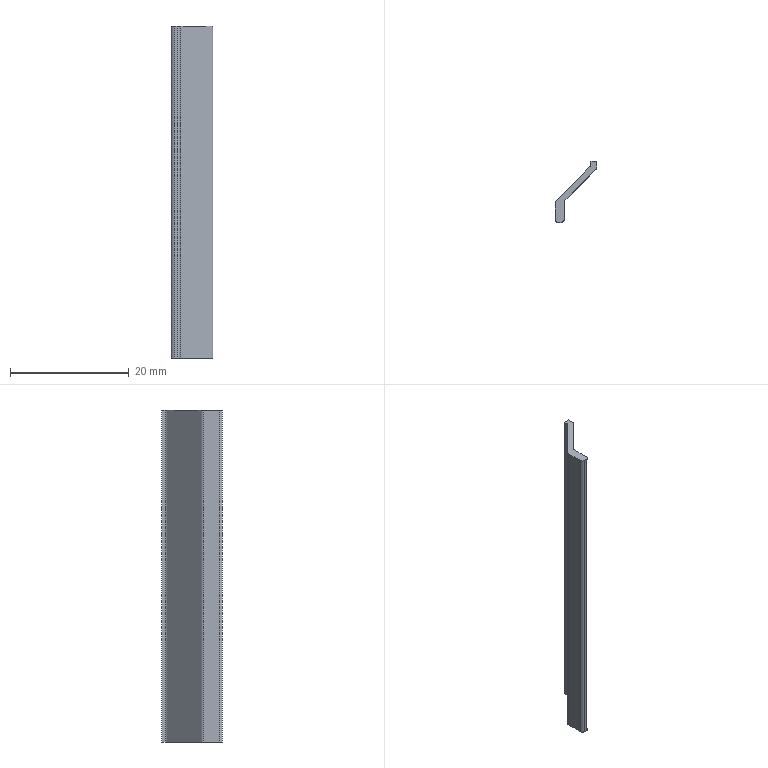Part | NX | features BREP 2 | 2 solids | 32 faces | box 7.015 x 10.276 x 56 mm | volume 1594 mm3 | plane 20 | cylinder 12 | commonest cylinder face diameters 1 x12
STEP:
#1=CARTESIAN_POINT('',(3.508,4.17,-4.));
#2=VERTEX_POINT('',#1);
#3=CARTESIAN_POINT('',(3.508,4.17,52.));
#4=VERTEX_POINT('',#3);
#5=CARTESIAN_POINT('',(3.508,4.17,0.));
#6=DIRECTION('',(0.,0.,1.));
#7=VECTOR('',#6,1000.);
#8=LINE('',#5,#7);
#9=EDGE_CURVE('',#2,#4,#8,.T.);
#10=ORIENTED_EDGE('',*,*,#9,.T.);
#11=CARTESIAN_POINT('',(3.361,3.817,52.));
#12=VERTEX_POINT('',#11);
#13=CARTESIAN_POINT('',(3.008,4.17,52.));
#14=DIRECTION('',(0.,0.,1.));
#15=DIRECTION('',(1.,0.,0.));
#16=AXIS2_PLACEMENT_3D('',#13,#14,#15);
#17=CIRCLE('',#16,0.5);
#18=EDGE_CURVE('',#12,#4,#17,.T.);
#19=ORIENTED_EDGE('',*,*,#18,.F.);
#20=CARTESIAN_POINT('',(3.361,3.817,-4.));
#21=VERTEX_POINT('',#20);
#22=CARTESIAN_POINT('',(3.361,3.817,0.));
#23=DIRECTION('',(0.,0.,1.));
#24=VECTOR('',#23,1000.);
#25=LINE('',#22,#24);
#26=EDGE_CURVE('',#21,#12,#25,.T.);
#27=ORIENTED_EDGE('',*,*,#26,.F.);
#28=CARTESIAN_POINT('',(3.008,4.17,-4.));
#29=DIRECTION('',(0.,0.,1.));
#30=DIRECTION('',(1.,0.,0.));
#31=AXIS2_PLACEMENT_3D('',#28,#29,#30);
#32=CIRCLE('',#31,0.5);
#33=EDGE_CURVE('',#21,#2,#32,.T.);
#34=ORIENTED_EDGE('',*,*,#33,.T.);
#35=EDGE_LOOP('',(#10,#19,#27,#34));
#36=FACE_BOUND('',#35,.T.);
#37=CARTESIAN_POINT('',(3.008,4.17,0.));
#38=DIRECTION('',(0.,0.,1.));
#39=DIRECTION('',(-1.,0.,0.));
#40=AXIS2_PLACEMENT_3D('',#37,#38,#39);
#41=CYLINDRICAL_SURFACE('',#40,0.5);
#42=ADVANCED_FACE('',(#36),#41,.T.);
#43=ORIENTED_EDGE('',*,*,#26,.T.);
#44=CARTESIAN_POINT('',(-1.861,-1.406,52.));
#45=VERTEX_POINT('',#44);
#46=CARTESIAN_POINT('',(3.361,3.817,52.));
#47=DIRECTION('',(0.7071,0.7071,0.));
#48=VECTOR('',#47,1000.);
#49=LINE('',#46,#48);
#50=EDGE_CURVE('',#45,#12,#49,.T.);
#51=ORIENTED_EDGE('',*,*,#50,.F.);
#52=CARTESIAN_POINT('',(-1.861,-1.406,-4.));
#53=VERTEX_POINT('',#52);
#54=CARTESIAN_POINT('',(-1.861,-1.406,0.));
#55=DIRECTION('',(0.,0.,1.));
#56=VECTOR('',#55,1000.);
#57=LINE('',#54,#56);
#58=EDGE_CURVE('',#53,#45,#57,.T.);
#59=ORIENTED_EDGE('',*,*,#58,.F.);
#60=CARTESIAN_POINT('',(3.361,3.817,-4.));
#61=DIRECTION('',(0.7071,0.7071,0.));
#62=VECTOR('',#61,1000.);
#63=LINE('',#60,#62);
#64=EDGE_CURVE('',#53,#21,#63,.T.);
#65=ORIENTED_EDGE('',*,*,#64,.T.);
#66=EDGE_LOOP('',(#43,#51,#59,#65));
#67=FACE_BOUND('',#66,.T.);
#68=CARTESIAN_POINT('',(3.361,3.817,0.));
#69=DIRECTION('',(-0.7071,0.7071,0.));
#70=DIRECTION('',(0.7071,0.7071,0.));
#71=AXIS2_PLACEMENT_3D('',#68,#69,#70);
#72=PLANE('',#71);
#73=ADVANCED_FACE('',(#67),#72,.F.);
#74=ORIENTED_EDGE('',*,*,#58,.T.);
#75=CARTESIAN_POINT('',(-2.008,-1.76,52.));
#76=VERTEX_POINT('',#75);
#77=CARTESIAN_POINT('',(-1.508,-1.76,52.));
#78=DIRECTION('',(0.,0.,-1.));
#79=DIRECTION('',(1.,0.,0.));
#80=AXIS2_PLACEMENT_3D('',#77,#78,#79);
#81=CIRCLE('',#80,0.5);
#82=EDGE_CURVE('',#76,#45,#81,.T.);
#83=ORIENTED_EDGE('',*,*,#82,.F.);
#84=CARTESIAN_POINT('',(-2.008,-1.76,-4.));
#85=VERTEX_POINT('',#84);
#86=CARTESIAN_POINT('',(-2.008,-1.76,0.));
#87=DIRECTION('',(0.,0.,1.));
#88=VECTOR('',#87,1000.);
#89=LINE('',#86,#88);
#90=EDGE_CURVE('',#85,#76,#89,.T.);
#91=ORIENTED_EDGE('',*,*,#90,.F.);
#92=CARTESIAN_POINT('',(-1.508,-1.76,-4.));
#93=DIRECTION('',(0.,0.,-1.));
#94=DIRECTION('',(1.,0.,0.));
#95=AXIS2_PLACEMENT_3D('',#92,#93,#94);
#96=CIRCLE('',#95,0.5);
#97=EDGE_CURVE('',#85,#53,#96,.T.);
#98=ORIENTED_EDGE('',*,*,#97,.T.);
#99=EDGE_LOOP('',(#74,#83,#91,#98));
#100=FACE_BOUND('',#99,.T.);
#101=CARTESIAN_POINT('',(-1.508,-1.76,0.));
#102=DIRECTION('',(0.,0.,1.));
#103=DIRECTION('',(-1.,0.,0.));
#104=AXIS2_PLACEMENT_3D('',#101,#102,#103);
#105=CYLINDRICAL_SURFACE('',#104,0.5);
#106=ADVANCED_FACE('',(#100),#105,.F.);
#107=ORIENTED_EDGE('',*,*,#90,.T.);
#108=CARTESIAN_POINT('',(-2.008,-4.613,52.));
#109=VERTEX_POINT('',#108);
#110=CARTESIAN_POINT('',(-2.008,-7.135,52.));
#111=DIRECTION('',(0.,1.,0.));
#112=VECTOR('',#111,1000.);
#113=LINE('',#110,#112);
#114=EDGE_CURVE('',#109,#76,#113,.T.);
#115=ORIENTED_EDGE('',*,*,#114,.F.);
#116=CARTESIAN_POINT('',(-2.008,-4.613,-4.));
#117=VERTEX_POINT('',#116);
#118=CARTESIAN_POINT('',(-2.008,-4.613,0.));
#119=DIRECTION('',(0.,0.,1.));
#120=VECTOR('',#119,1000.);
#121=LINE('',#118,#120);
#122=EDGE_CURVE('',#117,#109,#121,.T.);
#123=ORIENTED_EDGE('',*,*,#122,.F.);
#124=CARTESIAN_POINT('',(-2.008,-7.135,-4.));
#125=DIRECTION('',(0.,1.,0.));
#126=VECTOR('',#125,1000.);
#127=LINE('',#124,#126);
#128=EDGE_CURVE('',#117,#85,#127,.T.);
#129=ORIENTED_EDGE('',*,*,#128,.T.);
#130=EDGE_LOOP('',(#107,#115,#123,#129));
#131=FACE_BOUND('',#130,.T.);
#132=CARTESIAN_POINT('',(-2.008,-1.76,0.));
#133=DIRECTION('',(-1.,0.,0.));
#134=DIRECTION('',(0.,1.,0.));
#135=AXIS2_PLACEMENT_3D('',#132,#133,#134);
#136=PLANE('',#135);
#137=ADVANCED_FACE('',(#131),#136,.F.);
#138=ORIENTED_EDGE('',*,*,#122,.T.);
#139=CARTESIAN_POINT('',(-2.508,-5.113,52.));
#140=VERTEX_POINT('',#139);
#141=CARTESIAN_POINT('',(-2.508,-4.613,52.));
#142=DIRECTION('',(0.,0.,1.));
#143=DIRECTION('',(1.,0.,0.));
#144=AXIS2_PLACEMENT_3D('',#141,#142,#143);
#145=CIRCLE('',#144,0.5);
#146=EDGE_CURVE('',#140,#109,#145,.T.);
#147=ORIENTED_EDGE('',*,*,#146,.F.);
#148=CARTESIAN_POINT('',(-2.508,-5.113,-4.));
#149=VERTEX_POINT('',#148);
#150=CARTESIAN_POINT('',(-2.508,-5.113,0.));
#151=DIRECTION('',(0.,0.,1.));
#152=VECTOR('',#151,1000.);
#153=LINE('',#150,#152);
#154=EDGE_CURVE('',#149,#140,#153,.T.);
#155=ORIENTED_EDGE('',*,*,#154,.F.);
#156=CARTESIAN_POINT('',(-2.508,-4.613,-4.));
#157=DIRECTION('',(0.,0.,1.));
#158=DIRECTION('',(1.,0.,0.));
#159=AXIS2_PLACEMENT_3D('',#156,#157,#158);
#160=CIRCLE('',#159,0.5);
#161=EDGE_CURVE('',#149,#117,#160,.T.);
#162=ORIENTED_EDGE('',*,*,#161,.T.);
#163=EDGE_LOOP('',(#138,#147,#155,#162));
#164=FACE_BOUND('',#163,.T.);
#165=CARTESIAN_POINT('',(-2.508,-4.613,0.));
#166=DIRECTION('',(0.,0.,1.));
#167=DIRECTION('',(-1.,0.,0.));
#168=AXIS2_PLACEMENT_3D('',#165,#166,#167);
#169=CYLINDRICAL_SURFACE('',#168,0.5);
#170=ADVANCED_FACE('',(#164),#169,.T.);
#171=ORIENTED_EDGE('',*,*,#154,.T.);
#172=CARTESIAN_POINT('',(-3.008,-5.113,52.));
#173=VERTEX_POINT('',#172);
#174=CARTESIAN_POINT('',(-0.5343,-5.113,52.));
#175=DIRECTION('',(1.,0.,0.));
#176=VECTOR('',#175,1000.);
#177=LINE('',#174,#176);
#178=EDGE_CURVE('',#173,#140,#177,.T.);
#179=ORIENTED_EDGE('',*,*,#178,.F.);
#180=CARTESIAN_POINT('',(-3.008,-5.113,-4.));
#181=VERTEX_POINT('',#180);
#182=CARTESIAN_POINT('',(-3.008,-5.113,0.));
#183=DIRECTION('',(0.,0.,1.));
#184=VECTOR('',#183,1000.);
#185=LINE('',#182,#184);
#186=EDGE_CURVE('',#181,#173,#185,.T.);
#187=ORIENTED_EDGE('',*,*,#186,.F.);
#188=CARTESIAN_POINT('',(-0.5343,-5.113,-4.));
#189=DIRECTION('',(1.,0.,0.));
#190=VECTOR('',#189,1000.);
#191=LINE('',#188,#190);
#192=EDGE_CURVE('',#181,#149,#191,.T.);
#193=ORIENTED_EDGE('',*,*,#192,.T.);
#194=EDGE_LOOP('',(#171,#179,#187,#193));
#195=FACE_BOUND('',#194,.T.);
#196=CARTESIAN_POINT('',(-2.508,-5.113,0.));
#197=DIRECTION('',(0.,1.,0.));
#198=DIRECTION('',(1.,0.,0.));
#199=AXIS2_PLACEMENT_3D('',#196,#197,#198);
#200=PLANE('',#199);
#201=ADVANCED_FACE('',(#195),#200,.F.);
#202=ORIENTED_EDGE('',*,*,#186,.T.);
#203=CARTESIAN_POINT('',(-3.508,-4.613,52.));
#204=VERTEX_POINT('',#203);
#205=CARTESIAN_POINT('',(-3.008,-4.613,52.));
#206=DIRECTION('',(0.,0.,1.));
#207=DIRECTION('',(1.,0.,0.));
#208=AXIS2_PLACEMENT_3D('',#205,#206,#207);
#209=CIRCLE('',#208,0.5);
#210=EDGE_CURVE('',#204,#173,#209,.T.);
#211=ORIENTED_EDGE('',*,*,#210,.F.);
#212=CARTESIAN_POINT('',(-3.508,-4.613,-4.));
#213=VERTEX_POINT('',#212);
#214=CARTESIAN_POINT('',(-3.508,-4.613,0.));
#215=DIRECTION('',(0.,0.,1.));
#216=VECTOR('',#215,1000.);
#217=LINE('',#214,#216);
#218=EDGE_CURVE('',#213,#204,#217,.T.);
#219=ORIENTED_EDGE('',*,*,#218,.F.);
#220=CARTESIAN_POINT('',(-3.008,-4.613,-4.));
#221=DIRECTION('',(0.,0.,1.));
#222=DIRECTION('',(1.,0.,0.));
#223=AXIS2_PLACEMENT_3D('',#220,#221,#222);
#224=CIRCLE('',#223,0.5);
#225=EDGE_CURVE('',#213,#181,#224,.T.);
#226=ORIENTED_EDGE('',*,*,#225,.T.);
#227=EDGE_LOOP('',(#202,#211,#219,#226));
#228=FACE_BOUND('',#227,.T.);
#229=CARTESIAN_POINT('',(-3.008,-4.613,0.));
#230=DIRECTION('',(0.,0.,1.));
#231=DIRECTION('',(-1.,0.,0.));
#232=AXIS2_PLACEMENT_3D('',#229,#230,#231);
#233=CYLINDRICAL_SURFACE('',#232,0.5);
#234=ADVANCED_FACE('',(#228),#233,.T.);
#235=ORIENTED_EDGE('',*,*,#218,.T.);
#236=CARTESIAN_POINT('',(-3.508,-1.86,52.));
#237=VERTEX_POINT('',#236);
#238=CARTESIAN_POINT('',(-3.508,-7.135,52.));
#239=DIRECTION('',(0.,-1.,0.));
#240=VECTOR('',#239,1000.);
#241=LINE('',#238,#240);
#242=EDGE_CURVE('',#237,#204,#241,.T.);
#243=ORIENTED_EDGE('',*,*,#242,.F.);
#244=CARTESIAN_POINT('',(-3.508,-1.86,-4.));
#245=VERTEX_POINT('',#244);
#246=CARTESIAN_POINT('',(-3.508,-1.86,0.));
#247=DIRECTION('',(0.,0.,1.));
#248=VECTOR('',#247,1000.);
#249=LINE('',#246,#248);
#250=EDGE_CURVE('',#245,#237,#249,.T.);
#251=ORIENTED_EDGE('',*,*,#250,.F.);
#252=CARTESIAN_POINT('',(-3.508,-7.135,-4.));
#253=DIRECTION('',(0.,-1.,0.));
#254=VECTOR('',#253,1000.);
#255=LINE('',#252,#254);
#256=EDGE_CURVE('',#245,#213,#255,.T.);
#257=ORIENTED_EDGE('',*,*,#256,.T.);
#258=EDGE_LOOP('',(#235,#243,#251,#257));
#259=FACE_BOUND('',#258,.T.);
#260=CARTESIAN_POINT('',(-3.508,-4.613,0.));
#261=DIRECTION('',(1.,0.,0.));
#262=DIRECTION('',(0.,-1.,0.));
#263=AXIS2_PLACEMENT_3D('',#260,#261,#262);
#264=PLANE('',#263);
#265=ADVANCED_FACE('',(#259),#264,.F.);
#266=ORIENTED_EDGE('',*,*,#250,.T.);
#267=CARTESIAN_POINT('',(-3.361,-1.506,52.));
#268=VERTEX_POINT('',#267);
#269=CARTESIAN_POINT('',(-3.008,-1.86,52.));
#270=DIRECTION('',(0.,0.,1.));
#271=DIRECTION('',(1.,0.,0.));
#272=AXIS2_PLACEMENT_3D('',#269,#270,#271);
#273=CIRCLE('',#272,0.5);
#274=EDGE_CURVE('',#268,#237,#273,.T.);
#275=ORIENTED_EDGE('',*,*,#274,.F.);
#276=CARTESIAN_POINT('',(-3.361,-1.506,-4.));
#277=VERTEX_POINT('',#276);
#278=CARTESIAN_POINT('',(-3.361,-1.506,0.));
#279=DIRECTION('',(0.,0.,1.));
#280=VECTOR('',#279,1000.);
#281=LINE('',#278,#280);
#282=EDGE_CURVE('',#277,#268,#281,.T.);
#283=ORIENTED_EDGE('',*,*,#282,.F.);
#284=CARTESIAN_POINT('',(-3.008,-1.86,-4.));
#285=DIRECTION('',(0.,0.,1.));
#286=DIRECTION('',(1.,0.,0.));
#287=AXIS2_PLACEMENT_3D('',#284,#285,#286);
#288=CIRCLE('',#287,0.5);
#289=EDGE_CURVE('',#277,#245,#288,.T.);
#290=ORIENTED_EDGE('',*,*,#289,.T.);
#291=EDGE_LOOP('',(#266,#275,#283,#290));
#292=FACE_BOUND('',#291,.T.);
#293=CARTESIAN_POINT('',(-3.008,-1.86,0.));
#294=DIRECTION('',(0.,0.,1.));
#295=DIRECTION('',(-1.,0.,0.));
#296=AXIS2_PLACEMENT_3D('',#293,#294,#295);
#297=CYLINDRICAL_SURFACE('',#296,0.5);
#298=ADVANCED_FACE('',(#292),#297,.T.);
#299=ORIENTED_EDGE('',*,*,#282,.T.);
#300=CARTESIAN_POINT('',(2.361,4.217,52.));
#301=VERTEX_POINT('',#300);
#302=CARTESIAN_POINT('',(-3.361,-1.506,52.));
#303=DIRECTION('',(-0.7071,-0.7071,0.));
#304=VECTOR('',#303,1000.);
#305=LINE('',#302,#304);
#306=EDGE_CURVE('',#301,#268,#305,.T.);
#307=ORIENTED_EDGE('',*,*,#306,.F.);
#308=CARTESIAN_POINT('',(2.361,4.217,-4.));
#309=VERTEX_POINT('',#308);
#310=CARTESIAN_POINT('',(2.361,4.217,0.));
#311=DIRECTION('',(0.,0.,1.));
#312=VECTOR('',#311,1000.);
#313=LINE('',#310,#312);
#314=EDGE_CURVE('',#309,#301,#313,.T.);
#315=ORIENTED_EDGE('',*,*,#314,.F.);
#316=CARTESIAN_POINT('',(-3.361,-1.506,-4.));
#317=DIRECTION('',(-0.7071,-0.7071,0.));
#318=VECTOR('',#317,1000.);
#319=LINE('',#316,#318);
#320=EDGE_CURVE('',#309,#277,#319,.T.);
#321=ORIENTED_EDGE('',*,*,#320,.T.);
#322=EDGE_LOOP('',(#299,#307,#315,#321));
#323=FACE_BOUND('',#322,.T.);
#324=CARTESIAN_POINT('',(-3.361,-1.506,0.));
#325=DIRECTION('',(0.7071,-0.7071,0.));
#326=DIRECTION('',(-0.7071,-0.7071,0.));
#327=AXIS2_PLACEMENT_3D('',#324,#325,#326);
#328=PLANE('',#327);
#329=ADVANCED_FACE('',(#323),#328,.F.);
#330=ORIENTED_EDGE('',*,*,#314,.T.);
#331=CARTESIAN_POINT('',(2.508,4.57,52.));
#332=VERTEX_POINT('',#331);
#333=CARTESIAN_POINT('',(2.008,4.57,52.));
#334=DIRECTION('',(0.,0.,-1.));
#335=DIRECTION('',(1.,0.,0.));
#336=AXIS2_PLACEMENT_3D('',#333,#334,#335);
#337=CIRCLE('',#336,0.5);
#338=EDGE_CURVE('',#332,#301,#337,.T.);
#339=ORIENTED_EDGE('',*,*,#338,.F.);
#340=CARTESIAN_POINT('',(2.508,4.57,-4.));
#341=VERTEX_POINT('',#340);
#342=CARTESIAN_POINT('',(2.508,4.57,0.));
#343=DIRECTION('',(0.,0.,1.));
#344=VECTOR('',#343,1000.);
#345=LINE('',#342,#344);
#346=EDGE_CURVE('',#341,#332,#345,.T.);
#347=ORIENTED_EDGE('',*,*,#346,.F.);
#348=CARTESIAN_POINT('',(2.008,4.57,-4.));
#349=DIRECTION('',(0.,0.,-1.));
#350=DIRECTION('',(1.,0.,0.));
#351=AXIS2_PLACEMENT_3D('',#348,#349,#350);
#352=CIRCLE('',#351,0.5);
#353=EDGE_CURVE('',#341,#309,#352,.T.);
#354=ORIENTED_EDGE('',*,*,#353,.T.);
#355=EDGE_LOOP('',(#330,#339,#347,#354));
#356=FACE_BOUND('',#355,.T.);
#357=CARTESIAN_POINT('',(2.008,4.57,0.));
#358=DIRECTION('',(0.,0.,1.));
#359=DIRECTION('',(-1.,0.,0.));
#360=AXIS2_PLACEMENT_3D('',#357,#358,#359);
#361=CYLINDRICAL_SURFACE('',#360,0.5);
#362=ADVANCED_FACE('',(#356),#361,.F.);
#363=ORIENTED_EDGE('',*,*,#346,.T.);
#364=CARTESIAN_POINT('',(2.508,5.163,52.));
#365=VERTEX_POINT('',#364);
#366=CARTESIAN_POINT('',(2.508,-7.135,52.));
#367=DIRECTION('',(0.,-1.,0.));
#368=VECTOR('',#367,1000.);
#369=LINE('',#366,#368);
#370=EDGE_CURVE('',#365,#332,#369,.T.);
#371=ORIENTED_EDGE('',*,*,#370,.F.);
#372=CARTESIAN_POINT('',(2.508,5.163,-4.));
#373=VERTEX_POINT('',#372);
#374=CARTESIAN_POINT('',(2.508,5.163,0.));
#375=DIRECTION('',(0.,0.,1.));
#376=VECTOR('',#375,1000.);
#377=LINE('',#374,#376);
#378=EDGE_CURVE('',#373,#365,#377,.T.);
#379=ORIENTED_EDGE('',*,*,#378,.F.);
#380=CARTESIAN_POINT('',(2.508,-7.135,-4.));
#381=DIRECTION('',(0.,-1.,0.));
#382=VECTOR('',#381,1000.);
#383=LINE('',#380,#382);
#384=EDGE_CURVE('',#373,#341,#383,.T.);
#385=ORIENTED_EDGE('',*,*,#384,.T.);
#386=EDGE_LOOP('',(#363,#371,#379,#385));
#387=FACE_BOUND('',#386,.T.);
#388=CARTESIAN_POINT('',(2.508,4.57,0.));
#389=DIRECTION('',(1.,0.,0.));
#390=DIRECTION('',(0.,-1.,0.));
#391=AXIS2_PLACEMENT_3D('',#388,#389,#390);
#392=PLANE('',#391);
#393=ADVANCED_FACE('',(#387),#392,.F.);
#394=ORIENTED_EDGE('',*,*,#378,.T.);
#395=CARTESIAN_POINT('',(3.508,5.163,52.));
#396=VERTEX_POINT('',#395);
#397=CARTESIAN_POINT('',(-0.5343,5.163,52.));
#398=DIRECTION('',(-1.,0.,0.));
#399=VECTOR('',#398,1000.);
#400=LINE('',#397,#399);
#401=EDGE_CURVE('',#396,#365,#400,.T.);
#402=ORIENTED_EDGE('',*,*,#401,.F.);
#403=CARTESIAN_POINT('',(3.508,5.163,-4.));
#404=VERTEX_POINT('',#403);
#405=CARTESIAN_POINT('',(3.508,5.163,0.));
#406=DIRECTION('',(0.,0.,1.));
#407=VECTOR('',#406,1000.);
#408=LINE('',#405,#407);
#409=EDGE_CURVE('',#404,#396,#408,.T.);
#410=ORIENTED_EDGE('',*,*,#409,.F.);
#411=CARTESIAN_POINT('',(-0.5343,5.163,-4.));
#412=DIRECTION('',(-1.,0.,0.));
#413=VECTOR('',#412,1000.);
#414=LINE('',#411,#413);
#415=EDGE_CURVE('',#404,#373,#414,.T.);
#416=ORIENTED_EDGE('',*,*,#415,.T.);
#417=EDGE_LOOP('',(#394,#402,#410,#416));
#418=FACE_BOUND('',#417,.T.);
#419=CARTESIAN_POINT('',(-0.5343,5.163,0.));
#420=DIRECTION('',(0.,-1.,0.));
#421=DIRECTION('',(-1.,0.,0.));
#422=AXIS2_PLACEMENT_3D('',#419,#420,#421);
#423=PLANE('',#422);
#424=ADVANCED_FACE('',(#418),#423,.F.);
#425=CARTESIAN_POINT('',(3.508,-7.135,-4.));
#426=DIRECTION('',(0.,1.,0.));
#427=VECTOR('',#426,1000.);
#428=LINE('',#425,#427);
#429=EDGE_CURVE('',#2,#404,#428,.T.);
#430=ORIENTED_EDGE('',*,*,#429,.T.);
#431=ORIENTED_EDGE('',*,*,#409,.T.);
#432=CARTESIAN_POINT('',(3.508,-7.135,52.));
#433=DIRECTION('',(0.,1.,0.));
#434=VECTOR('',#433,1000.);
#435=LINE('',#432,#434);
#436=EDGE_CURVE('',#4,#396,#435,.T.);
#437=ORIENTED_EDGE('',*,*,#436,.F.);
#438=ORIENTED_EDGE('',*,*,#9,.F.);
#439=EDGE_LOOP('',(#430,#431,#437,#438));
#440=FACE_BOUND('',#439,.T.);
#441=CARTESIAN_POINT('',(3.508,10.163,0.));
#442=DIRECTION('',(-1.,0.,0.));
#443=DIRECTION('',(0.,1.,0.));
#444=AXIS2_PLACEMENT_3D('',#441,#442,#443);
#445=PLANE('',#444);
#446=ADVANCED_FACE('',(#440),#445,.F.);
#447=ORIENTED_EDGE('',*,*,#401,.T.);
#448=ORIENTED_EDGE('',*,*,#370,.T.);
#449=ORIENTED_EDGE('',*,*,#338,.T.);
#450=ORIENTED_EDGE('',*,*,#306,.T.);
#451=ORIENTED_EDGE('',*,*,#274,.T.);
#452=ORIENTED_EDGE('',*,*,#242,.T.);
#453=ORIENTED_EDGE('',*,*,#210,.T.);
#454=ORIENTED_EDGE('',*,*,#178,.T.);
#455=ORIENTED_EDGE('',*,*,#146,.T.);
#456=ORIENTED_EDGE('',*,*,#114,.T.);
#457=ORIENTED_EDGE('',*,*,#82,.T.);
#458=ORIENTED_EDGE('',*,*,#50,.T.);
#459=ORIENTED_EDGE('',*,*,#18,.T.);
#460=ORIENTED_EDGE('',*,*,#436,.T.);
#461=EDGE_LOOP('',(#447,#448,#449,#450,#451,#452,#453,#454,#455,#456,#457,#458,#459,#460));
#462=FACE_BOUND('',#461,.T.);
#463=CARTESIAN_POINT('',(-0.5343,-7.135,52.));
#464=DIRECTION('',(0.,0.,1.));
#465=DIRECTION('',(-1.,0.,0.));
#466=AXIS2_PLACEMENT_3D('',#463,#464,#465);
#467=PLANE('',#466);
#468=ADVANCED_FACE('',(#462),#467,.T.);
#469=ORIENTED_EDGE('',*,*,#415,.F.);
#470=ORIENTED_EDGE('',*,*,#429,.F.);
#471=ORIENTED_EDGE('',*,*,#33,.F.);
#472=ORIENTED_EDGE('',*,*,#64,.F.);
#473=ORIENTED_EDGE('',*,*,#97,.F.);
#474=ORIENTED_EDGE('',*,*,#128,.F.);
#475=ORIENTED_EDGE('',*,*,#161,.F.);
#476=ORIENTED_EDGE('',*,*,#192,.F.);
#477=ORIENTED_EDGE('',*,*,#225,.F.);
#478=ORIENTED_EDGE('',*,*,#256,.F.);
#479=ORIENTED_EDGE('',*,*,#289,.F.);
#480=ORIENTED_EDGE('',*,*,#320,.F.);
#481=ORIENTED_EDGE('',*,*,#353,.F.);
#482=ORIENTED_EDGE('',*,*,#384,.F.);
#483=EDGE_LOOP('',(#469,#470,#471,#472,#473,#474,#475,#476,#477,#478,#479,#480,#481,#482));
#484=FACE_BOUND('',#483,.T.);
#485=CARTESIAN_POINT('',(-0.5343,-7.135,-4.));
#486=DIRECTION('',(0.,0.,1.));
#487=DIRECTION('',(-1.,0.,0.));
#488=AXIS2_PLACEMENT_3D('',#485,#486,#487);
#489=PLANE('',#488);
#490=ADVANCED_FACE('',(#484),#489,.F.);
#491=CLOSED_SHELL('',(#42,#73,#106,#137,#170,#201,#234,#265,#298,#329,#362,#393,#424,#446,#468,#490));
#492=MANIFOLD_SOLID_BREP('',#491);
#493=CARTESIAN_POINT('',(3.508,4.17,-4.));
#494=VERTEX_POINT('',#493);
#495=CARTESIAN_POINT('',(3.508,4.17,52.));
#496=VERTEX_POINT('',#495);
#497=CARTESIAN_POINT('',(3.508,4.17,0.));
#498=DIRECTION('',(0.,0.,1.));
#499=VECTOR('',#498,1000.);
#500=LINE('',#497,#499);
#501=EDGE_CURVE('',#494,#496,#500,.T.);
#502=ORIENTED_EDGE('',*,*,#501,.T.);
#503=CARTESIAN_POINT('',(3.361,3.817,52.));
#504=VERTEX_POINT('',#503);
#505=CARTESIAN_POINT('',(3.008,4.17,52.));
#506=DIRECTION('',(0.,0.,1.));
#507=DIRECTION('',(1.,0.,0.));
#508=AXIS2_PLACEMENT_3D('',#505,#506,#507);
#509=CIRCLE('',#508,0.5);
#510=EDGE_CURVE('',#504,#496,#509,.T.);
#511=ORIENTED_EDGE('',*,*,#510,.F.);
#512=CARTESIAN_POINT('',(3.361,3.817,-4.));
#513=VERTEX_POINT('',#512);
#514=CARTESIAN_POINT('',(3.361,3.817,0.));
#515=DIRECTION('',(0.,0.,1.));
#516=VECTOR('',#515,1000.);
#517=LINE('',#514,#516);
#518=EDGE_CURVE('',#513,#504,#517,.T.);
#519=ORIENTED_EDGE('',*,*,#518,.F.);
#520=CARTESIAN_POINT('',(3.008,4.17,-4.));
#521=DIRECTION('',(0.,0.,1.));
#522=DIRECTION('',(1.,0.,0.));
#523=AXIS2_PLACEMENT_3D('',#520,#521,#522);
#524=CIRCLE('',#523,0.5);
#525=EDGE_CURVE('',#513,#494,#524,.T.);
#526=ORIENTED_EDGE('',*,*,#525,.T.);
#527=EDGE_LOOP('',(#502,#511,#519,#526));
#528=FACE_BOUND('',#527,.T.);
#529=CARTESIAN_POINT('',(3.008,4.17,0.));
#530=DIRECTION('',(0.,0.,1.));
#531=DIRECTION('',(-1.,0.,0.));
#532=AXIS2_PLACEMENT_3D('',#529,#530,#531);
#533=CYLINDRICAL_SURFACE('',#532,0.5);
#534=ADVANCED_FACE('',(#528),#533,.T.);
#535=ORIENTED_EDGE('',*,*,#518,.T.);
#536=CARTESIAN_POINT('',(-1.861,-1.406,52.));
#537=VERTEX_POINT('',#536);
#538=CARTESIAN_POINT('',(3.361,3.817,52.));
#539=DIRECTION('',(0.7071,0.7071,0.));
#540=VECTOR('',#539,1000.);
#541=LINE('',#538,#540);
#542=EDGE_CURVE('',#537,#504,#541,.T.);
#543=ORIENTED_EDGE('',*,*,#542,.F.);
#544=CARTESIAN_POINT('',(-1.861,-1.406,-4.));
#545=VERTEX_POINT('',#544);
#546=CARTESIAN_POINT('',(-1.861,-1.406,0.));
#547=DIRECTION('',(0.,0.,1.));
#548=VECTOR('',#547,1000.);
#549=LINE('',#546,#548);
#550=EDGE_CURVE('',#545,#537,#549,.T.);
#551=ORIENTED_EDGE('',*,*,#550,.F.);
#552=CARTESIAN_POINT('',(3.361,3.817,-4.));
#553=DIRECTION('',(0.7071,0.7071,0.));
#554=VECTOR('',#553,1000.);
#555=LINE('',#552,#554);
#556=EDGE_CURVE('',#545,#513,#555,.T.);
#557=ORIENTED_EDGE('',*,*,#556,.T.);
#558=EDGE_LOOP('',(#535,#543,#551,#557));
#559=FACE_BOUND('',#558,.T.);
#560=CARTESIAN_POINT('',(3.361,3.817,0.));
#561=DIRECTION('',(-0.7071,0.7071,0.));
#562=DIRECTION('',(0.7071,0.7071,0.));
#563=AXIS2_PLACEMENT_3D('',#560,#561,#562);
#564=PLANE('',#563);
#565=ADVANCED_FACE('',(#559),#564,.F.);
#566=ORIENTED_EDGE('',*,*,#550,.T.);
#567=CARTESIAN_POINT('',(-2.008,-1.76,52.));
#568=VERTEX_POINT('',#567);
#569=CARTESIAN_POINT('',(-1.508,-1.76,52.));
#570=DIRECTION('',(0.,0.,-1.));
#571=DIRECTION('',(1.,0.,0.));
#572=AXIS2_PLACEMENT_3D('',#569,#570,#571);
#573=CIRCLE('',#572,0.5);
#574=EDGE_CURVE('',#568,#537,#573,.T.);
#575=ORIENTED_EDGE('',*,*,#574,.F.);
#576=CARTESIAN_POINT('',(-2.008,-1.76,-4.));
#577=VERTEX_POINT('',#576);
#578=CARTESIAN_POINT('',(-2.008,-1.76,0.));
#579=DIRECTION('',(0.,0.,1.));
#580=VECTOR('',#579,1000.);
#581=LINE('',#578,#580);
#582=EDGE_CURVE('',#577,#568,#581,.T.);
#583=ORIENTED_EDGE('',*,*,#582,.F.);
#584=CARTESIAN_POINT('',(-1.508,-1.76,-4.));
#585=DIRECTION('',(0.,0.,-1.));
#586=DIRECTION('',(1.,0.,0.));
#587=AXIS2_PLACEMENT_3D('',#584,#585,#586);
#588=CIRCLE('',#587,0.5);
#589=EDGE_CURVE('',#577,#545,#588,.T.);
#590=ORIENTED_EDGE('',*,*,#589,.T.);
#591=EDGE_LOOP('',(#566,#575,#583,#590));
#592=FACE_BOUND('',#591,.T.);
#593=CARTESIAN_POINT('',(-1.508,-1.76,0.));
#594=DIRECTION('',(0.,0.,1.));
#595=DIRECTION('',(-1.,0.,0.));
#596=AXIS2_PLACEMENT_3D('',#593,#594,#595);
#597=CYLINDRICAL_SURFACE('',#596,0.5);
#598=ADVANCED_FACE('',(#592),#597,.F.);
#599=ORIENTED_EDGE('',*,*,#582,.T.);
#600=CARTESIAN_POINT('',(-2.008,-4.613,52.));
#601=VERTEX_POINT('',#600);
#602=CARTESIAN_POINT('',(-2.008,-7.135,52.));
#603=DIRECTION('',(0.,1.,0.));
#604=VECTOR('',#603,1000.);
#605=LINE('',#602,#604);
#606=EDGE_CURVE('',#601,#568,#605,.T.);
#607=ORIENTED_EDGE('',*,*,#606,.F.);
#608=CARTESIAN_POINT('',(-2.008,-4.613,-4.));
#609=VERTEX_POINT('',#608);
#610=CARTESIAN_POINT('',(-2.008,-4.613,0.));
#611=DIRECTION('',(0.,0.,1.));
#612=VECTOR('',#611,1000.);
#613=LINE('',#610,#612);
#614=EDGE_CURVE('',#609,#601,#613,.T.);
#615=ORIENTED_EDGE('',*,*,#614,.F.);
#616=CARTESIAN_POINT('',(-2.008,-7.135,-4.));
#617=DIRECTION('',(0.,1.,0.));
#618=VECTOR('',#617,1000.);
#619=LINE('',#616,#618);
#620=EDGE_CURVE('',#609,#577,#619,.T.);
#621=ORIENTED_EDGE('',*,*,#620,.T.);
#622=EDGE_LOOP('',(#599,#607,#615,#621));
#623=FACE_BOUND('',#622,.T.);
#624=CARTESIAN_POINT('',(-2.008,-1.76,0.));
#625=DIRECTION('',(-1.,0.,0.));
#626=DIRECTION('',(0.,1.,0.));
#627=AXIS2_PLACEMENT_3D('',#624,#625,#626);
#628=PLANE('',#627);
#629=ADVANCED_FACE('',(#623),#628,.F.);
#630=ORIENTED_EDGE('',*,*,#614,.T.);
#631=CARTESIAN_POINT('',(-2.508,-5.113,52.));
#632=VERTEX_POINT('',#631);
#633=CARTESIAN_POINT('',(-2.508,-4.613,52.));
#634=DIRECTION('',(0.,0.,1.));
#635=DIRECTION('',(1.,0.,0.));
#636=AXIS2_PLACEMENT_3D('',#633,#634,#635);
#637=CIRCLE('',#636,0.5);
#638=EDGE_CURVE('',#632,#601,#637,.T.);
#639=ORIENTED_EDGE('',*,*,#638,.F.);
#640=CARTESIAN_POINT('',(-2.508,-5.113,-4.));
#641=VERTEX_POINT('',#640);
#642=CARTESIAN_POINT('',(-2.508,-5.113,0.));
#643=DIRECTION('',(0.,0.,1.));
#644=VECTOR('',#643,1000.);
#645=LINE('',#642,#644);
#646=EDGE_CURVE('',#641,#632,#645,.T.);
#647=ORIENTED_EDGE('',*,*,#646,.F.);
#648=CARTESIAN_POINT('',(-2.508,-4.613,-4.));
#649=DIRECTION('',(0.,0.,1.));
#650=DIRECTION('',(1.,0.,0.));
#651=AXIS2_PLACEMENT_3D('',#648,#649,#650);
#652=CIRCLE('',#651,0.5);
#653=EDGE_CURVE('',#641,#609,#652,.T.);
#654=ORIENTED_EDGE('',*,*,#653,.T.);
#655=EDGE_LOOP('',(#630,#639,#647,#654));
#656=FACE_BOUND('',#655,.T.);
#657=CARTESIAN_POINT('',(-2.508,-4.613,0.));
#658=DIRECTION('',(0.,0.,1.));
#659=DIRECTION('',(-1.,0.,0.));
#660=AXIS2_PLACEMENT_3D('',#657,#658,#659);
#661=CYLINDRICAL_SURFACE('',#660,0.5);
#662=ADVANCED_FACE('',(#656),#661,.T.);
#663=ORIENTED_EDGE('',*,*,#646,.T.);
#664=CARTESIAN_POINT('',(-3.008,-5.113,52.));
#665=VERTEX_POINT('',#664);
#666=CARTESIAN_POINT('',(-0.5343,-5.113,52.));
#667=DIRECTION('',(1.,0.,0.));
#668=VECTOR('',#667,1000.);
#669=LINE('',#666,#668);
#670=EDGE_CURVE('',#665,#632,#669,.T.);
#671=ORIENTED_EDGE('',*,*,#670,.F.);
#672=CARTESIAN_POINT('',(-3.008,-5.113,-4.));
#673=VERTEX_POINT('',#672);
#674=CARTESIAN_POINT('',(-3.008,-5.113,0.));
#675=DIRECTION('',(0.,0.,1.));
#676=VECTOR('',#675,1000.);
#677=LINE('',#674,#676);
#678=EDGE_CURVE('',#673,#665,#677,.T.);
#679=ORIENTED_EDGE('',*,*,#678,.F.);
#680=CARTESIAN_POINT('',(-0.5343,-5.113,-4.));
#681=DIRECTION('',(1.,0.,0.));
#682=VECTOR('',#681,1000.);
#683=LINE('',#680,#682);
#684=EDGE_CURVE('',#673,#641,#683,.T.);
#685=ORIENTED_EDGE('',*,*,#684,.T.);
#686=EDGE_LOOP('',(#663,#671,#679,#685));
#687=FACE_BOUND('',#686,.T.);
#688=CARTESIAN_POINT('',(-2.508,-5.113,0.));
#689=DIRECTION('',(0.,1.,0.));
#690=DIRECTION('',(1.,0.,0.));
#691=AXIS2_PLACEMENT_3D('',#688,#689,#690);
#692=PLANE('',#691);
#693=ADVANCED_FACE('',(#687),#692,.F.);
#694=ORIENTED_EDGE('',*,*,#678,.T.);
#695=CARTESIAN_POINT('',(-3.508,-4.613,52.));
#696=VERTEX_POINT('',#695);
#697=CARTESIAN_POINT('',(-3.008,-4.613,52.));
#698=DIRECTION('',(0.,0.,1.));
#699=DIRECTION('',(1.,0.,0.));
#700=AXIS2_PLACEMENT_3D('',#697,#698,#699);
#701=CIRCLE('',#700,0.5);
#702=EDGE_CURVE('',#696,#665,#701,.T.);
#703=ORIENTED_EDGE('',*,*,#702,.F.);
#704=CARTESIAN_POINT('',(-3.508,-4.613,-4.));
#705=VERTEX_POINT('',#704);
#706=CARTESIAN_POINT('',(-3.508,-4.613,0.));
#707=DIRECTION('',(0.,0.,1.));
#708=VECTOR('',#707,1000.);
#709=LINE('',#706,#708);
#710=EDGE_CURVE('',#705,#696,#709,.T.);
#711=ORIENTED_EDGE('',*,*,#710,.F.);
#712=CARTESIAN_POINT('',(-3.008,-4.613,-4.));
#713=DIRECTION('',(0.,0.,1.));
#714=DIRECTION('',(1.,0.,0.));
#715=AXIS2_PLACEMENT_3D('',#712,#713,#714);
#716=CIRCLE('',#715,0.5);
#717=EDGE_CURVE('',#705,#673,#716,.T.);
#718=ORIENTED_EDGE('',*,*,#717,.T.);
#719=EDGE_LOOP('',(#694,#703,#711,#718));
#720=FACE_BOUND('',#719,.T.);
#721=CARTESIAN_POINT('',(-3.008,-4.613,0.));
#722=DIRECTION('',(0.,0.,1.));
#723=DIRECTION('',(-1.,0.,0.));
#724=AXIS2_PLACEMENT_3D('',#721,#722,#723);
#725=CYLINDRICAL_SURFACE('',#724,0.5);
#726=ADVANCED_FACE('',(#720),#725,.T.);
#727=ORIENTED_EDGE('',*,*,#710,.T.);
#728=CARTESIAN_POINT('',(-3.508,-1.86,52.));
#729=VERTEX_POINT('',#728);
#730=CARTESIAN_POINT('',(-3.508,-7.135,52.));
#731=DIRECTION('',(0.,-1.,0.));
#732=VECTOR('',#731,1000.);
#733=LINE('',#730,#732);
#734=EDGE_CURVE('',#729,#696,#733,.T.);
#735=ORIENTED_EDGE('',*,*,#734,.F.);
#736=CARTESIAN_POINT('',(-3.508,-1.86,-4.));
#737=VERTEX_POINT('',#736);
#738=CARTESIAN_POINT('',(-3.508,-1.86,0.));
#739=DIRECTION('',(0.,0.,1.));
#740=VECTOR('',#739,1000.);
#741=LINE('',#738,#740);
#742=EDGE_CURVE('',#737,#729,#741,.T.);
#743=ORIENTED_EDGE('',*,*,#742,.F.);
#744=CARTESIAN_POINT('',(-3.508,-7.135,-4.));
#745=DIRECTION('',(0.,-1.,0.));
#746=VECTOR('',#745,1000.);
#747=LINE('',#744,#746);
#748=EDGE_CURVE('',#737,#705,#747,.T.);
#749=ORIENTED_EDGE('',*,*,#748,.T.);
#750=EDGE_LOOP('',(#727,#735,#743,#749));
#751=FACE_BOUND('',#750,.T.);
#752=CARTESIAN_POINT('',(-3.508,-4.613,0.));
#753=DIRECTION('',(1.,0.,0.));
#754=DIRECTION('',(0.,-1.,0.));
#755=AXIS2_PLACEMENT_3D('',#752,#753,#754);
#756=PLANE('',#755);
#757=ADVANCED_FACE('',(#751),#756,.F.);
#758=ORIENTED_EDGE('',*,*,#742,.T.);
#759=CARTESIAN_POINT('',(-3.361,-1.506,52.));
#760=VERTEX_POINT('',#759);
#761=CARTESIAN_POINT('',(-3.008,-1.86,52.));
#762=DIRECTION('',(0.,0.,1.));
#763=DIRECTION('',(1.,0.,0.));
#764=AXIS2_PLACEMENT_3D('',#761,#762,#763);
#765=CIRCLE('',#764,0.5);
#766=EDGE_CURVE('',#760,#729,#765,.T.);
#767=ORIENTED_EDGE('',*,*,#766,.F.);
#768=CARTESIAN_POINT('',(-3.361,-1.506,-4.));
#769=VERTEX_POINT('',#768);
#770=CARTESIAN_POINT('',(-3.361,-1.506,0.));
#771=DIRECTION('',(0.,0.,1.));
#772=VECTOR('',#771,1000.);
#773=LINE('',#770,#772);
#774=EDGE_CURVE('',#769,#760,#773,.T.);
#775=ORIENTED_EDGE('',*,*,#774,.F.);
#776=CARTESIAN_POINT('',(-3.008,-1.86,-4.));
#777=DIRECTION('',(0.,0.,1.));
#778=DIRECTION('',(1.,0.,0.));
#779=AXIS2_PLACEMENT_3D('',#776,#777,#778);
#780=CIRCLE('',#779,0.5);
#781=EDGE_CURVE('',#769,#737,#780,.T.);
#782=ORIENTED_EDGE('',*,*,#781,.T.);
#783=EDGE_LOOP('',(#758,#767,#775,#782));
#784=FACE_BOUND('',#783,.T.);
#785=CARTESIAN_POINT('',(-3.008,-1.86,0.));
#786=DIRECTION('',(0.,0.,1.));
#787=DIRECTION('',(-1.,0.,0.));
#788=AXIS2_PLACEMENT_3D('',#785,#786,#787);
#789=CYLINDRICAL_SURFACE('',#788,0.5);
#790=ADVANCED_FACE('',(#784),#789,.T.);
#791=ORIENTED_EDGE('',*,*,#774,.T.);
#792=CARTESIAN_POINT('',(2.361,4.217,52.));
#793=VERTEX_POINT('',#792);
#794=CARTESIAN_POINT('',(-3.361,-1.506,52.));
#795=DIRECTION('',(-0.7071,-0.7071,0.));
#796=VECTOR('',#795,1000.);
#797=LINE('',#794,#796);
#798=EDGE_CURVE('',#793,#760,#797,.T.);
#799=ORIENTED_EDGE('',*,*,#798,.F.);
#800=CARTESIAN_POINT('',(2.361,4.217,-4.));
#801=VERTEX_POINT('',#800);
#802=CARTESIAN_POINT('',(2.361,4.217,0.));
#803=DIRECTION('',(0.,0.,1.));
#804=VECTOR('',#803,1000.);
#805=LINE('',#802,#804);
#806=EDGE_CURVE('',#801,#793,#805,.T.);
#807=ORIENTED_EDGE('',*,*,#806,.F.);
#808=CARTESIAN_POINT('',(-3.361,-1.506,-4.));
#809=DIRECTION('',(-0.7071,-0.7071,0.));
#810=VECTOR('',#809,1000.);
#811=LINE('',#808,#810);
#812=EDGE_CURVE('',#801,#769,#811,.T.);
#813=ORIENTED_EDGE('',*,*,#812,.T.);
#814=EDGE_LOOP('',(#791,#799,#807,#813));
#815=FACE_BOUND('',#814,.T.);
#816=CARTESIAN_POINT('',(-3.361,-1.506,0.));
#817=DIRECTION('',(0.7071,-0.7071,0.));
#818=DIRECTION('',(-0.7071,-0.7071,0.));
#819=AXIS2_PLACEMENT_3D('',#816,#817,#818);
#820=PLANE('',#819);
#821=ADVANCED_FACE('',(#815),#820,.F.);
#822=ORIENTED_EDGE('',*,*,#806,.T.);
#823=CARTESIAN_POINT('',(2.508,4.57,52.));
#824=VERTEX_POINT('',#823);
#825=CARTESIAN_POINT('',(2.008,4.57,52.));
#826=DIRECTION('',(0.,0.,-1.));
#827=DIRECTION('',(1.,0.,0.));
#828=AXIS2_PLACEMENT_3D('',#825,#826,#827);
#829=CIRCLE('',#828,0.5);
#830=EDGE_CURVE('',#824,#793,#829,.T.);
#831=ORIENTED_EDGE('',*,*,#830,.F.);
#832=CARTESIAN_POINT('',(2.508,4.57,-4.));
#833=VERTEX_POINT('',#832);
#834=CARTESIAN_POINT('',(2.508,4.57,0.));
#835=DIRECTION('',(0.,0.,1.));
#836=VECTOR('',#835,1000.);
#837=LINE('',#834,#836);
#838=EDGE_CURVE('',#833,#824,#837,.T.);
#839=ORIENTED_EDGE('',*,*,#838,.F.);
#840=CARTESIAN_POINT('',(2.008,4.57,-4.));
#841=DIRECTION('',(0.,0.,-1.));
#842=DIRECTION('',(1.,0.,0.));
#843=AXIS2_PLACEMENT_3D('',#840,#841,#842);
#844=CIRCLE('',#843,0.5);
#845=EDGE_CURVE('',#833,#801,#844,.T.);
#846=ORIENTED_EDGE('',*,*,#845,.T.);
#847=EDGE_LOOP('',(#822,#831,#839,#846));
#848=FACE_BOUND('',#847,.T.);
#849=CARTESIAN_POINT('',(2.008,4.57,0.));
#850=DIRECTION('',(0.,0.,1.));
#851=DIRECTION('',(-1.,0.,0.));
#852=AXIS2_PLACEMENT_3D('',#849,#850,#851);
#853=CYLINDRICAL_SURFACE('',#852,0.5);
#854=ADVANCED_FACE('',(#848),#853,.F.);
#855=ORIENTED_EDGE('',*,*,#838,.T.);
#856=CARTESIAN_POINT('',(2.508,5.163,52.));
#857=VERTEX_POINT('',#856);
#858=CARTESIAN_POINT('',(2.508,-7.135,52.));
#859=DIRECTION('',(0.,-1.,0.));
#860=VECTOR('',#859,1000.);
#861=LINE('',#858,#860);
#862=EDGE_CURVE('',#857,#824,#861,.T.);
#863=ORIENTED_EDGE('',*,*,#862,.F.);
#864=CARTESIAN_POINT('',(2.508,5.163,-4.));
#865=VERTEX_POINT('',#864);
#866=CARTESIAN_POINT('',(2.508,5.163,0.));
#867=DIRECTION('',(0.,0.,1.));
#868=VECTOR('',#867,1000.);
#869=LINE('',#866,#868);
#870=EDGE_CURVE('',#865,#857,#869,.T.);
#871=ORIENTED_EDGE('',*,*,#870,.F.);
#872=CARTESIAN_POINT('',(2.508,-7.135,-4.));
#873=DIRECTION('',(0.,-1.,0.));
#874=VECTOR('',#873,1000.);
#875=LINE('',#872,#874);
#876=EDGE_CURVE('',#865,#833,#875,.T.);
#877=ORIENTED_EDGE('',*,*,#876,.T.);
#878=EDGE_LOOP('',(#855,#863,#871,#877));
#879=FACE_BOUND('',#878,.T.);
#880=CARTESIAN_POINT('',(2.508,4.57,0.));
#881=DIRECTION('',(1.,0.,0.));
#882=DIRECTION('',(0.,-1.,0.));
#883=AXIS2_PLACEMENT_3D('',#880,#881,#882);
#884=PLANE('',#883);
#885=ADVANCED_FACE('',(#879),#884,.F.);
#886=ORIENTED_EDGE('',*,*,#870,.T.);
#887=CARTESIAN_POINT('',(3.508,5.163,52.));
#888=VERTEX_POINT('',#887);
#889=CARTESIAN_POINT('',(-0.5343,5.163,52.));
#890=DIRECTION('',(-1.,0.,0.));
#891=VECTOR('',#890,1000.);
#892=LINE('',#889,#891);
#893=EDGE_CURVE('',#888,#857,#892,.T.);
#894=ORIENTED_EDGE('',*,*,#893,.F.);
#895=CARTESIAN_POINT('',(3.508,5.163,-4.));
#896=VERTEX_POINT('',#895);
#897=CARTESIAN_POINT('',(3.508,5.163,0.));
#898=DIRECTION('',(0.,0.,1.));
#899=VECTOR('',#898,1000.);
#900=LINE('',#897,#899);
#901=EDGE_CURVE('',#896,#888,#900,.T.);
#902=ORIENTED_EDGE('',*,*,#901,.F.);
#903=CARTESIAN_POINT('',(-0.5343,5.163,-4.));
#904=DIRECTION('',(-1.,0.,0.));
#905=VECTOR('',#904,1000.);
#906=LINE('',#903,#905);
#907=EDGE_CURVE('',#896,#865,#906,.T.);
#908=ORIENTED_EDGE('',*,*,#907,.T.);
#909=EDGE_LOOP('',(#886,#894,#902,#908));
#910=FACE_BOUND('',#909,.T.);
#911=CARTESIAN_POINT('',(-0.5343,5.163,0.));
#912=DIRECTION('',(0.,-1.,0.));
#913=DIRECTION('',(-1.,0.,0.));
#914=AXIS2_PLACEMENT_3D('',#911,#912,#913);
#915=PLANE('',#914);
#916=ADVANCED_FACE('',(#910),#915,.F.);
#917=CARTESIAN_POINT('',(3.508,-7.135,-4.));
#918=DIRECTION('',(0.,1.,0.));
#919=VECTOR('',#918,1000.);
#920=LINE('',#917,#919);
#921=EDGE_CURVE('',#494,#896,#920,.T.);
#922=ORIENTED_EDGE('',*,*,#921,.T.);
#923=ORIENTED_EDGE('',*,*,#901,.T.);
#924=CARTESIAN_POINT('',(3.508,-7.135,52.));
#925=DIRECTION('',(0.,1.,0.));
#926=VECTOR('',#925,1000.);
#927=LINE('',#924,#926);
#928=EDGE_CURVE('',#496,#888,#927,.T.);
#929=ORIENTED_EDGE('',*,*,#928,.F.);
#930=ORIENTED_EDGE('',*,*,#501,.F.);
#931=EDGE_LOOP('',(#922,#923,#929,#930));
#932=FACE_BOUND('',#931,.T.);
#933=CARTESIAN_POINT('',(3.508,10.163,0.));
#934=DIRECTION('',(-1.,0.,0.));
#935=DIRECTION('',(0.,1.,0.));
#936=AXIS2_PLACEMENT_3D('',#933,#934,#935);
#937=PLANE('',#936);
#938=ADVANCED_FACE('',(#932),#937,.F.);
#939=ORIENTED_EDGE('',*,*,#893,.T.);
#940=ORIENTED_EDGE('',*,*,#862,.T.);
#941=ORIENTED_EDGE('',*,*,#830,.T.);
#942=ORIENTED_EDGE('',*,*,#798,.T.);
#943=ORIENTED_EDGE('',*,*,#766,.T.);
#944=ORIENTED_EDGE('',*,*,#734,.T.);
#945=ORIENTED_EDGE('',*,*,#702,.T.);
#946=ORIENTED_EDGE('',*,*,#670,.T.);
#947=ORIENTED_EDGE('',*,*,#638,.T.);
#948=ORIENTED_EDGE('',*,*,#606,.T.);
#949=ORIENTED_EDGE('',*,*,#574,.T.);
#950=ORIENTED_EDGE('',*,*,#542,.T.);
#951=ORIENTED_EDGE('',*,*,#510,.T.);
#952=ORIENTED_EDGE('',*,*,#928,.T.);
#953=EDGE_LOOP('',(#939,#940,#941,#942,#943,#944,#945,#946,#947,#948,#949,#950,#951,#952));
#954=FACE_BOUND('',#953,.T.);
#955=CARTESIAN_POINT('',(-0.5343,-7.135,52.));
#956=DIRECTION('',(0.,0.,1.));
#957=DIRECTION('',(-1.,0.,0.));
#958=AXIS2_PLACEMENT_3D('',#955,#956,#957);
#959=PLANE('',#958);
#960=ADVANCED_FACE('',(#954),#959,.T.);
#961=ORIENTED_EDGE('',*,*,#907,.F.);
#962=ORIENTED_EDGE('',*,*,#921,.F.);
#963=ORIENTED_EDGE('',*,*,#525,.F.);
#964=ORIENTED_EDGE('',*,*,#556,.F.);
#965=ORIENTED_EDGE('',*,*,#589,.F.);
#966=ORIENTED_EDGE('',*,*,#620,.F.);
#967=ORIENTED_EDGE('',*,*,#653,.F.);
#968=ORIENTED_EDGE('',*,*,#684,.F.);
#969=ORIENTED_EDGE('',*,*,#717,.F.);
#970=ORIENTED_EDGE('',*,*,#748,.F.);
#971=ORIENTED_EDGE('',*,*,#781,.F.);
#972=ORIENTED_EDGE('',*,*,#812,.F.);
#973=ORIENTED_EDGE('',*,*,#845,.F.);
#974=ORIENTED_EDGE('',*,*,#876,.F.);
#975=EDGE_LOOP('',(#961,#962,#963,#964,#965,#966,#967,#968,#969,#970,#971,#972,#973,#974));
#976=FACE_BOUND('',#975,.T.);
#977=CARTESIAN_POINT('',(-0.5343,-7.135,-4.));
#978=DIRECTION('',(0.,0.,1.));
#979=DIRECTION('',(-1.,0.,0.));
#980=AXIS2_PLACEMENT_3D('',#977,#978,#979);
#981=PLANE('',#980);
#982=ADVANCED_FACE('',(#976),#981,.F.);
#983=CLOSED_SHELL('',(#534,#565,#598,#629,#662,#693,#726,#757,#790,#821,#854,#885,#916,#938,#960,#982));
#984=MANIFOLD_SOLID_BREP('',#983);
#985=(LENGTH_UNIT()NAMED_UNIT(*)SI_UNIT(.MILLI.,.METRE.));
#986=UNCERTAINTY_MEASURE_WITH_UNIT(LENGTH_MEASURE(0.00001),#985,'','');
#987=(NAMED_UNIT(*)PLANE_ANGLE_UNIT()SI_UNIT($,.RADIAN.));
#988=(NAMED_UNIT(*)SI_UNIT($,.STERADIAN.)SOLID_ANGLE_UNIT());
#989=(GEOMETRIC_REPRESENTATION_CONTEXT(3)GLOBAL_UNCERTAINTY_ASSIGNED_CONTEXT((#986))GLOBAL_UNIT_ASSIGNED_CONTEXT((#985,#987,#988))REPRESENTATION_CONTEXT('',''));
#990=ADVANCED_BREP_SHAPE_REPRESENTATION('',(#492,#984),#989);